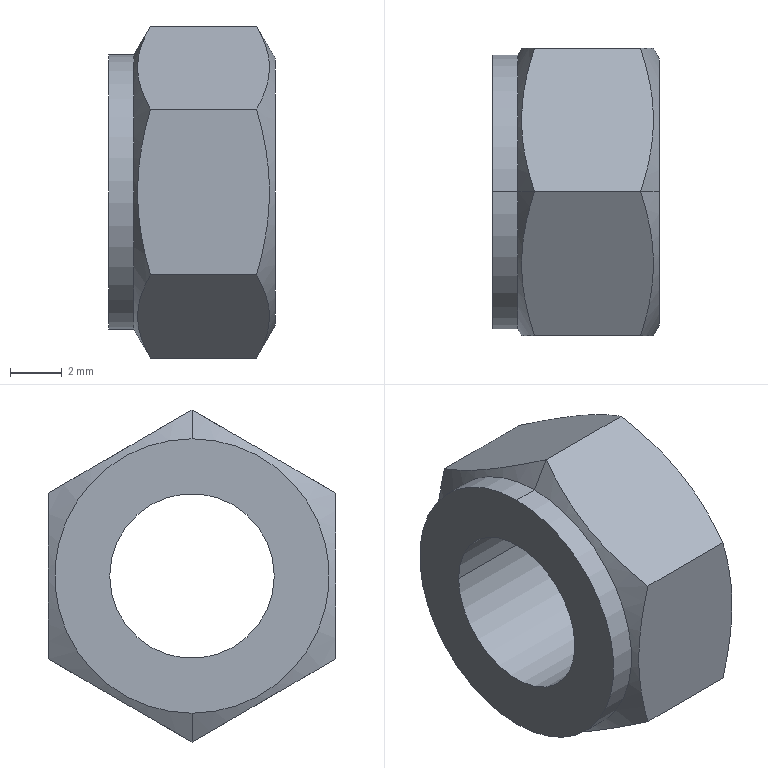Part | NX | features BREP 1 | 1 solid | 16 faces | box 6.426 x 11.1 x 12.817 mm | volume 455.339 mm3 | plane 8 | cylinder 4 | cone 4 | commonest cylinder face diameters 6.35 x2 10.592 x2
STEP:
#1=CARTESIAN_POINT('',(5.537,0.,5.159));
#2=VERTEX_POINT('',#1);
#3=CARTESIAN_POINT('',(5.537,0.,-5.159));
#4=VERTEX_POINT('',#3);
#5=CARTESIAN_POINT('',(5.537,0.,0.));
#6=DIRECTION('',(-1.,0.,0.));
#7=DIRECTION('',(0.,0.,1.));
#8=AXIS2_PLACEMENT_3D('',#5,#6,#7);
#9=CIRCLE('',#8,5.159);
#10=EDGE_CURVE('',#2,#4,#9,.T.);
#11=ORIENTED_EDGE('',*,*,#10,.F.);
#12=CARTESIAN_POINT('',(5.537,0.,0.));
#13=DIRECTION('',(-1.,0.,0.));
#14=DIRECTION('',(0.,0.,-1.));
#15=AXIS2_PLACEMENT_3D('',#12,#13,#14);
#16=CIRCLE('',#15,5.159);
#17=EDGE_CURVE('',#4,#2,#16,.T.);
#18=ORIENTED_EDGE('',*,*,#17,.F.);
#19=EDGE_LOOP('',(#11,#18));
#20=FACE_BOUND('',#19,.T.);
#21=CARTESIAN_POINT('',(5.537,-3.175,0.));
#22=VERTEX_POINT('',#21);
#23=CARTESIAN_POINT('',(5.537,3.175,0.));
#24=VERTEX_POINT('',#23);
#25=CARTESIAN_POINT('',(5.537,0.,0.));
#26=DIRECTION('',(1.,0.,0.));
#27=DIRECTION('',(0.,-1.,0.));
#28=AXIS2_PLACEMENT_3D('',#25,#26,#27);
#29=CIRCLE('',#28,3.175);
#30=EDGE_CURVE('',#22,#24,#29,.T.);
#31=ORIENTED_EDGE('',*,*,#30,.F.);
#32=CARTESIAN_POINT('',(5.537,0.,0.));
#33=DIRECTION('',(1.,0.,0.));
#34=DIRECTION('',(0.,1.,0.));
#35=AXIS2_PLACEMENT_3D('',#32,#33,#34);
#36=CIRCLE('',#35,3.175);
#37=EDGE_CURVE('',#24,#22,#36,.T.);
#38=ORIENTED_EDGE('',*,*,#37,.F.);
#39=EDGE_LOOP('',(#31,#38));
#40=FACE_BOUND('',#39,.T.);
#41=CARTESIAN_POINT('',(5.537,0.,0.));
#42=DIRECTION('',(1.,0.,0.));
#43=DIRECTION('',(0.,1.,0.));
#44=AXIS2_PLACEMENT_3D('',#41,#42,#43);
#45=PLANE('',#44);
#46=ADVANCED_FACE('',(#20,#40),#45,.T.);
#47=ORIENTED_EDGE('',*,*,#37,.T.);
#48=CARTESIAN_POINT('',(-0.889,-3.175,0.));
#49=VERTEX_POINT('',#48);
#50=CARTESIAN_POINT('',(-0.889,-3.175,0.));
#51=DIRECTION('',(1.,0.,0.));
#52=VECTOR('',#51,1000.);
#53=LINE('',#50,#52);
#54=EDGE_CURVE('',#22,#49,#53,.F.);
#55=ORIENTED_EDGE('',*,*,#54,.T.);
#56=CARTESIAN_POINT('',(-0.889,3.175,0.));
#57=VERTEX_POINT('',#56);
#58=CARTESIAN_POINT('',(-0.889,0.,0.));
#59=DIRECTION('',(1.,0.,0.));
#60=DIRECTION('',(0.,1.,0.));
#61=AXIS2_PLACEMENT_3D('',#58,#59,#60);
#62=CIRCLE('',#61,3.175);
#63=EDGE_CURVE('',#57,#49,#62,.T.);
#64=ORIENTED_EDGE('',*,*,#63,.F.);
#65=CARTESIAN_POINT('',(-0.889,3.175,0.));
#66=DIRECTION('',(1.,0.,0.));
#67=VECTOR('',#66,1000.);
#68=LINE('',#65,#67);
#69=EDGE_CURVE('',#24,#57,#68,.F.);
#70=ORIENTED_EDGE('',*,*,#69,.F.);
#71=EDGE_LOOP('',(#47,#55,#64,#70));
#72=FACE_BOUND('',#71,.T.);
#73=CARTESIAN_POINT('',(-1.532,0.,0.));
#74=DIRECTION('',(1.,0.,0.));
#75=DIRECTION('',(0.,1.,0.));
#76=AXIS2_PLACEMENT_3D('',#73,#74,#75);
#77=CYLINDRICAL_SURFACE('',#76,3.175);
#78=ADVANCED_FACE('',(#72),#77,.F.);
#79=CARTESIAN_POINT('',(-0.889,0.,0.));
#80=DIRECTION('',(1.,0.,0.));
#81=DIRECTION('',(0.,-1.,0.));
#82=AXIS2_PLACEMENT_3D('',#79,#80,#81);
#83=CIRCLE('',#82,3.175);
#84=EDGE_CURVE('',#49,#57,#83,.T.);
#85=ORIENTED_EDGE('',*,*,#84,.F.);
#86=ORIENTED_EDGE('',*,*,#54,.F.);
#87=ORIENTED_EDGE('',*,*,#30,.T.);
#88=ORIENTED_EDGE('',*,*,#69,.T.);
#89=EDGE_LOOP('',(#85,#86,#87,#88));
#90=FACE_BOUND('',#89,.T.);
#91=CARTESIAN_POINT('',(-1.532,0.,0.));
#92=DIRECTION('',(1.,0.,0.));
#93=DIRECTION('',(0.,1.,0.));
#94=AXIS2_PLACEMENT_3D('',#91,#92,#93);
#95=CYLINDRICAL_SURFACE('',#94,3.175);
#96=ADVANCED_FACE('',(#90),#95,.F.);
#97=CARTESIAN_POINT('',(-0.889,0.,5.296));
#98=VERTEX_POINT('',#97);
#99=CARTESIAN_POINT('',(-0.889,0.,-5.296));
#100=VERTEX_POINT('',#99);
#101=CARTESIAN_POINT('',(-0.889,0.,0.));
#102=DIRECTION('',(-1.,0.,0.));
#103=DIRECTION('',(0.,0.,1.));
#104=AXIS2_PLACEMENT_3D('',#101,#102,#103);
#105=CIRCLE('',#104,5.296);
#106=EDGE_CURVE('',#98,#100,#105,.T.);
#107=ORIENTED_EDGE('',*,*,#106,.T.);
#108=CARTESIAN_POINT('',(-0.889,0.,0.));
#109=DIRECTION('',(-1.,0.,0.));
#110=DIRECTION('',(0.,0.,-1.));
#111=AXIS2_PLACEMENT_3D('',#108,#109,#110);
#112=CIRCLE('',#111,5.296);
#113=EDGE_CURVE('',#100,#98,#112,.T.);
#114=ORIENTED_EDGE('',*,*,#113,.T.);
#115=EDGE_LOOP('',(#107,#114));
#116=FACE_BOUND('',#115,.T.);
#117=ORIENTED_EDGE('',*,*,#84,.T.);
#118=ORIENTED_EDGE('',*,*,#63,.T.);
#119=EDGE_LOOP('',(#117,#118));
#120=FACE_BOUND('',#119,.T.);
#121=CARTESIAN_POINT('',(-0.889,0.,0.));
#122=DIRECTION('',(-1.,0.,0.));
#123=DIRECTION('',(0.,0.,1.));
#124=AXIS2_PLACEMENT_3D('',#121,#122,#123);
#125=PLANE('',#124);
#126=ADVANCED_FACE('',(#116,#120),#125,.T.);
#127=CARTESIAN_POINT('',(0.07914,0.,5.296));
#128=VERTEX_POINT('',#127);
#129=CARTESIAN_POINT('',(0.07914,0.,5.296));
#130=DIRECTION('',(-1.,0.,0.));
#131=VECTOR('',#130,1000.);
#132=LINE('',#129,#131);
#133=EDGE_CURVE('',#98,#128,#132,.F.);
#134=ORIENTED_EDGE('',*,*,#133,.F.);
#135=ORIENTED_EDGE('',*,*,#113,.F.);
#136=CARTESIAN_POINT('',(0.07914,0.,-5.296));
#137=VERTEX_POINT('',#136);
#138=CARTESIAN_POINT('',(0.07914,0.,-5.296));
#139=DIRECTION('',(-1.,0.,0.));
#140=VECTOR('',#139,1000.);
#141=LINE('',#138,#140);
#142=EDGE_CURVE('',#100,#137,#141,.F.);
#143=ORIENTED_EDGE('',*,*,#142,.T.);
#144=CARTESIAN_POINT('',(0.07914,0.,0.));
#145=DIRECTION('',(-1.,0.,0.));
#146=DIRECTION('',(0.,0.,-1.));
#147=AXIS2_PLACEMENT_3D('',#144,#145,#146);
#148=CIRCLE('',#147,5.296);
#149=EDGE_CURVE('',#137,#128,#148,.T.);
#150=ORIENTED_EDGE('',*,*,#149,.T.);
#151=EDGE_LOOP('',(#134,#135,#143,#150));
#152=FACE_BOUND('',#151,.T.);
#153=CARTESIAN_POINT('',(0.508,0.,0.));
#154=DIRECTION('',(-1.,0.,0.));
#155=DIRECTION('',(0.,0.,-1.));
#156=AXIS2_PLACEMENT_3D('',#153,#154,#155);
#157=CYLINDRICAL_SURFACE('',#156,5.296);
#158=ADVANCED_FACE('',(#152),#157,.T.);
#159=CARTESIAN_POINT('',(0.7215,0.,-6.408));
#160=VERTEX_POINT('',#159);
#161=CARTESIAN_POINT('',(0.07914,0.,-5.296));
#162=DIRECTION('',(0.5,0.,-0.866));
#163=VECTOR('',#162,1000.);
#164=LINE('',#161,#163);
#165=EDGE_CURVE('',#137,#160,#164,.T.);
#166=ORIENTED_EDGE('',*,*,#165,.T.);
#167=CARTESIAN_POINT('',(0.7215,-5.55,-3.204));
#168=VERTEX_POINT('',#167);
#169=CARTESIAN_POINT('',(0.7215,-5.55,-3.204));
#170=CARTESIAN_POINT('',(0.06136,-3.57,-4.348));
#171=CARTESIAN_POINT('',(0.06077,-1.982,-5.264));
#172=CARTESIAN_POINT('',(0.7215,0.,-6.408));
#173=B_SPLINE_CURVE_WITH_KNOTS('',3,(#169,#170,#171,#172),.UNSPECIFIED.,.F.,.F.,(4,4),(0.,1.),.UNSPECIFIED.);
#174=EDGE_CURVE('',#160,#168,#173,.F.);
#175=ORIENTED_EDGE('',*,*,#174,.T.);
#176=CARTESIAN_POINT('',(0.7215,-5.55,3.204));
#177=VERTEX_POINT('',#176);
#178=CARTESIAN_POINT('',(0.7215,-5.55,3.204));
#179=CARTESIAN_POINT('',(0.06136,-5.55,0.9175));
#180=CARTESIAN_POINT('',(0.06077,-5.55,-0.9155));
#181=CARTESIAN_POINT('',(0.7215,-5.55,-3.204));
#182=B_SPLINE_CURVE_WITH_KNOTS('',3,(#178,#179,#180,#181),.UNSPECIFIED.,.F.,.F.,(4,4),(0.,1.),.UNSPECIFIED.);
#183=EDGE_CURVE('',#168,#177,#182,.F.);
#184=ORIENTED_EDGE('',*,*,#183,.T.);
#185=CARTESIAN_POINT('',(0.7215,0.,6.408));
#186=VERTEX_POINT('',#185);
#187=CARTESIAN_POINT('',(0.7215,0.,6.408));
#188=CARTESIAN_POINT('',(0.06136,-1.98,5.265));
#189=CARTESIAN_POINT('',(0.06077,-3.568,4.349));
#190=CARTESIAN_POINT('',(0.7215,-5.55,3.204));
#191=B_SPLINE_CURVE_WITH_KNOTS('',3,(#187,#188,#189,#190),.UNSPECIFIED.,.F.,.F.,(4,4),(0.,1.),.UNSPECIFIED.);
#192=EDGE_CURVE('',#177,#186,#191,.F.);
#193=ORIENTED_EDGE('',*,*,#192,.T.);
#194=CARTESIAN_POINT('',(0.07914,0.,5.296));
#195=DIRECTION('',(0.5,0.,0.866));
#196=VECTOR('',#195,1000.);
#197=LINE('',#194,#196);
#198=EDGE_CURVE('',#128,#186,#197,.T.);
#199=ORIENTED_EDGE('',*,*,#198,.F.);
#200=ORIENTED_EDGE('',*,*,#149,.F.);
#201=EDGE_LOOP('',(#166,#175,#184,#193,#199,#200));
#202=FACE_BOUND('',#201,.T.);
#203=CARTESIAN_POINT('',(0.4003,0.,0.));
#204=DIRECTION('',(1.,0.,0.));
#205=DIRECTION('',(0.,0.,1.));
#206=AXIS2_PLACEMENT_3D('',#203,#204,#205);
#207=CONICAL_SURFACE('',#206,5.852,1.047);
#208=ADVANCED_FACE('',(#202),#207,.T.);
#209=ORIENTED_EDGE('',*,*,#198,.T.);
#210=CARTESIAN_POINT('',(0.7215,5.55,3.204));
#211=VERTEX_POINT('',#210);
#212=CARTESIAN_POINT('',(0.7215,5.55,3.204));
#213=CARTESIAN_POINT('',(0.06136,3.57,4.348));
#214=CARTESIAN_POINT('',(0.06077,1.982,5.264));
#215=CARTESIAN_POINT('',(0.7215,0.,6.408));
#216=B_SPLINE_CURVE_WITH_KNOTS('',3,(#212,#213,#214,#215),.UNSPECIFIED.,.F.,.F.,(4,4),(0.,1.),.UNSPECIFIED.);
#217=EDGE_CURVE('',#186,#211,#216,.F.);
#218=ORIENTED_EDGE('',*,*,#217,.T.);
#219=CARTESIAN_POINT('',(0.7215,5.55,-3.204));
#220=VERTEX_POINT('',#219);
#221=CARTESIAN_POINT('',(0.7215,5.55,-3.204));
#222=CARTESIAN_POINT('',(0.06136,5.55,-0.9175));
#223=CARTESIAN_POINT('',(0.06077,5.55,0.9155));
#224=CARTESIAN_POINT('',(0.7215,5.55,3.204));
#225=B_SPLINE_CURVE_WITH_KNOTS('',3,(#221,#222,#223,#224),.UNSPECIFIED.,.F.,.F.,(4,4),(0.,1.),.UNSPECIFIED.);
#226=EDGE_CURVE('',#211,#220,#225,.F.);
#227=ORIENTED_EDGE('',*,*,#226,.T.);
#228=CARTESIAN_POINT('',(0.7215,0.,-6.408));
#229=CARTESIAN_POINT('',(0.06136,1.98,-5.265));
#230=CARTESIAN_POINT('',(0.06077,3.568,-4.349));
#231=CARTESIAN_POINT('',(0.7215,5.55,-3.204));
#232=B_SPLINE_CURVE_WITH_KNOTS('',3,(#228,#229,#230,#231),.UNSPECIFIED.,.F.,.F.,(4,4),(0.,1.),.UNSPECIFIED.);
#233=EDGE_CURVE('',#220,#160,#232,.F.);
#234=ORIENTED_EDGE('',*,*,#233,.T.);
#235=ORIENTED_EDGE('',*,*,#165,.F.);
#236=CARTESIAN_POINT('',(0.07914,0.,0.));
#237=DIRECTION('',(-1.,0.,0.));
#238=DIRECTION('',(0.,0.,1.));
#239=AXIS2_PLACEMENT_3D('',#236,#237,#238);
#240=CIRCLE('',#239,5.296);
#241=EDGE_CURVE('',#128,#137,#240,.T.);
#242=ORIENTED_EDGE('',*,*,#241,.F.);
#243=EDGE_LOOP('',(#209,#218,#227,#234,#235,#242));
#244=FACE_BOUND('',#243,.T.);
#245=CARTESIAN_POINT('',(0.4003,0.,0.));
#246=DIRECTION('',(1.,0.,0.));
#247=DIRECTION('',(0.,0.,1.));
#248=AXIS2_PLACEMENT_3D('',#245,#246,#247);
#249=CONICAL_SURFACE('',#248,5.852,1.047);
#250=ADVANCED_FACE('',(#244),#249,.T.);
#251=ORIENTED_EDGE('',*,*,#142,.F.);
#252=ORIENTED_EDGE('',*,*,#106,.F.);
#253=ORIENTED_EDGE('',*,*,#133,.T.);
#254=ORIENTED_EDGE('',*,*,#241,.T.);
#255=EDGE_LOOP('',(#251,#252,#253,#254));
#256=FACE_BOUND('',#255,.T.);
#257=CARTESIAN_POINT('',(0.508,0.,0.));
#258=DIRECTION('',(-1.,0.,0.));
#259=DIRECTION('',(0.,0.,-1.));
#260=AXIS2_PLACEMENT_3D('',#257,#258,#259);
#261=CYLINDRICAL_SURFACE('',#260,5.296);
#262=ADVANCED_FACE('',(#256),#261,.T.);
#263=CARTESIAN_POINT('',(4.816,0.,-6.408));
#264=VERTEX_POINT('',#263);
#265=CARTESIAN_POINT('',(0.7215,0.,-6.408));
#266=DIRECTION('',(1.,0.,0.));
#267=VECTOR('',#266,1000.);
#268=LINE('',#265,#267);
#269=EDGE_CURVE('',#160,#264,#268,.T.);
#270=ORIENTED_EDGE('',*,*,#269,.F.);
#271=ORIENTED_EDGE('',*,*,#233,.F.);
#272=CARTESIAN_POINT('',(4.816,5.55,-3.204));
#273=VERTEX_POINT('',#272);
#274=CARTESIAN_POINT('',(0.7215,5.55,-3.204));
#275=DIRECTION('',(1.,0.,0.));
#276=VECTOR('',#275,1000.);
#277=LINE('',#274,#276);
#278=EDGE_CURVE('',#220,#273,#277,.T.);
#279=ORIENTED_EDGE('',*,*,#278,.T.);
#280=CARTESIAN_POINT('',(4.816,5.55,-3.204));
#281=CARTESIAN_POINT('',(5.476,3.57,-4.348));
#282=CARTESIAN_POINT('',(5.477,1.982,-5.264));
#283=CARTESIAN_POINT('',(4.816,0.,-6.408));
#284=B_SPLINE_CURVE_WITH_KNOTS('',3,(#280,#281,#282,#283),.UNSPECIFIED.,.F.,.F.,(4,4),(0.,1.),.UNSPECIFIED.);
#285=EDGE_CURVE('',#273,#264,#284,.T.);
#286=ORIENTED_EDGE('',*,*,#285,.T.);
#287=EDGE_LOOP('',(#270,#271,#279,#286));
#288=FACE_BOUND('',#287,.T.);
#289=CARTESIAN_POINT('',(0.,0.,-6.408));
#290=DIRECTION('',(0.,0.5,-0.866));
#291=DIRECTION('',(-1.,0.,0.));
#292=AXIS2_PLACEMENT_3D('',#289,#290,#291);
#293=PLANE('',#292);
#294=ADVANCED_FACE('',(#288),#293,.T.);
#295=CARTESIAN_POINT('',(5.537,0.,-5.159));
#296=DIRECTION('',(-0.5,0.,-0.866));
#297=VECTOR('',#296,1000.);
#298=LINE('',#295,#297);
#299=EDGE_CURVE('',#4,#264,#298,.T.);
#300=ORIENTED_EDGE('',*,*,#299,.T.);
#301=ORIENTED_EDGE('',*,*,#285,.F.);
#302=CARTESIAN_POINT('',(4.816,5.55,3.204));
#303=VERTEX_POINT('',#302);
#304=CARTESIAN_POINT('',(4.816,5.55,3.204));
#305=CARTESIAN_POINT('',(5.476,5.55,0.9175));
#306=CARTESIAN_POINT('',(5.477,5.55,-0.9151));
#307=CARTESIAN_POINT('',(4.816,5.55,-3.204));
#308=B_SPLINE_CURVE_WITH_KNOTS('',3,(#304,#305,#306,#307),.UNSPECIFIED.,.F.,.F.,(4,4),(0.,1.),.UNSPECIFIED.);
#309=EDGE_CURVE('',#303,#273,#308,.T.);
#310=ORIENTED_EDGE('',*,*,#309,.F.);
#311=CARTESIAN_POINT('',(4.816,0.,6.408));
#312=VERTEX_POINT('',#311);
#313=CARTESIAN_POINT('',(4.816,0.,6.408));
#314=CARTESIAN_POINT('',(5.476,1.98,5.265));
#315=CARTESIAN_POINT('',(5.477,3.567,4.349));
#316=CARTESIAN_POINT('',(4.816,5.55,3.204));
#317=B_SPLINE_CURVE_WITH_KNOTS('',3,(#313,#314,#315,#316),.UNSPECIFIED.,.F.,.F.,(4,4),(0.,1.),.UNSPECIFIED.);
#318=EDGE_CURVE('',#312,#303,#317,.T.);
#319=ORIENTED_EDGE('',*,*,#318,.F.);
#320=CARTESIAN_POINT('',(5.537,0.,5.159));
#321=DIRECTION('',(-0.5,0.,0.866));
#322=VECTOR('',#321,1000.);
#323=LINE('',#320,#322);
#324=EDGE_CURVE('',#2,#312,#323,.T.);
#325=ORIENTED_EDGE('',*,*,#324,.F.);
#326=ORIENTED_EDGE('',*,*,#10,.T.);
#327=EDGE_LOOP('',(#300,#301,#310,#319,#325,#326));
#328=FACE_BOUND('',#327,.T.);
#329=CARTESIAN_POINT('',(5.176,0.,0.));
#330=DIRECTION('',(-1.,0.,0.));
#331=DIRECTION('',(0.,0.,-1.));
#332=AXIS2_PLACEMENT_3D('',#329,#330,#331);
#333=CONICAL_SURFACE('',#332,5.784,1.047);
#334=ADVANCED_FACE('',(#328),#333,.T.);
#335=ORIENTED_EDGE('',*,*,#324,.T.);
#336=CARTESIAN_POINT('',(4.816,-5.55,3.204));
#337=VERTEX_POINT('',#336);
#338=CARTESIAN_POINT('',(4.816,-5.55,3.204));
#339=CARTESIAN_POINT('',(5.476,-3.57,4.348));
#340=CARTESIAN_POINT('',(5.477,-1.982,5.264));
#341=CARTESIAN_POINT('',(4.816,0.,6.408));
#342=B_SPLINE_CURVE_WITH_KNOTS('',3,(#338,#339,#340,#341),.UNSPECIFIED.,.F.,.F.,(4,4),(0.,1.),.UNSPECIFIED.);
#343=EDGE_CURVE('',#337,#312,#342,.T.);
#344=ORIENTED_EDGE('',*,*,#343,.F.);
#345=CARTESIAN_POINT('',(4.816,-5.55,-3.204));
#346=VERTEX_POINT('',#345);
#347=CARTESIAN_POINT('',(4.816,-5.55,-3.204));
#348=CARTESIAN_POINT('',(5.476,-5.55,-0.9175));
#349=CARTESIAN_POINT('',(5.477,-5.55,0.9151));
#350=CARTESIAN_POINT('',(4.816,-5.55,3.204));
#351=B_SPLINE_CURVE_WITH_KNOTS('',3,(#347,#348,#349,#350),.UNSPECIFIED.,.F.,.F.,(4,4),(0.,1.),.UNSPECIFIED.);
#352=EDGE_CURVE('',#346,#337,#351,.T.);
#353=ORIENTED_EDGE('',*,*,#352,.F.);
#354=CARTESIAN_POINT('',(4.816,0.,-6.408));
#355=CARTESIAN_POINT('',(5.476,-1.98,-5.265));
#356=CARTESIAN_POINT('',(5.477,-3.567,-4.349));
#357=CARTESIAN_POINT('',(4.816,-5.55,-3.204));
#358=B_SPLINE_CURVE_WITH_KNOTS('',3,(#354,#355,#356,#357),.UNSPECIFIED.,.F.,.F.,(4,4),(0.,1.),.UNSPECIFIED.);
#359=EDGE_CURVE('',#264,#346,#358,.T.);
#360=ORIENTED_EDGE('',*,*,#359,.F.);
#361=ORIENTED_EDGE('',*,*,#299,.F.);
#362=ORIENTED_EDGE('',*,*,#17,.T.);
#363=EDGE_LOOP('',(#335,#344,#353,#360,#361,#362));
#364=FACE_BOUND('',#363,.T.);
#365=CARTESIAN_POINT('',(5.176,0.,0.));
#366=DIRECTION('',(-1.,0.,0.));
#367=DIRECTION('',(0.,0.,-1.));
#368=AXIS2_PLACEMENT_3D('',#365,#366,#367);
#369=CONICAL_SURFACE('',#368,5.784,1.047);
#370=ADVANCED_FACE('',(#364),#369,.T.);
#371=CARTESIAN_POINT('',(0.7215,-5.55,-3.204));
#372=DIRECTION('',(1.,0.,0.));
#373=VECTOR('',#372,1000.);
#374=LINE('',#371,#373);
#375=EDGE_CURVE('',#168,#346,#374,.T.);
#376=ORIENTED_EDGE('',*,*,#375,.F.);
#377=ORIENTED_EDGE('',*,*,#174,.F.);
#378=ORIENTED_EDGE('',*,*,#269,.T.);
#379=ORIENTED_EDGE('',*,*,#359,.T.);
#380=EDGE_LOOP('',(#376,#377,#378,#379));
#381=FACE_BOUND('',#380,.T.);
#382=CARTESIAN_POINT('',(0.,-5.55,-3.204));
#383=DIRECTION('',(0.,-0.5,-0.866));
#384=DIRECTION('',(0.,-0.866,0.5));
#385=AXIS2_PLACEMENT_3D('',#382,#383,#384);
#386=PLANE('',#385);
#387=ADVANCED_FACE('',(#381),#386,.T.);
#388=CARTESIAN_POINT('',(0.7215,-5.55,3.204));
#389=DIRECTION('',(1.,0.,0.));
#390=VECTOR('',#389,1000.);
#391=LINE('',#388,#390);
#392=EDGE_CURVE('',#177,#337,#391,.T.);
#393=ORIENTED_EDGE('',*,*,#392,.F.);
#394=ORIENTED_EDGE('',*,*,#183,.F.);
#395=ORIENTED_EDGE('',*,*,#375,.T.);
#396=ORIENTED_EDGE('',*,*,#352,.T.);
#397=EDGE_LOOP('',(#393,#394,#395,#396));
#398=FACE_BOUND('',#397,.T.);
#399=CARTESIAN_POINT('',(0.,-5.55,3.204));
#400=DIRECTION('',(0.,-1.,0.));
#401=DIRECTION('',(0.,0.,-1.));
#402=AXIS2_PLACEMENT_3D('',#399,#400,#401);
#403=PLANE('',#402);
#404=ADVANCED_FACE('',(#398),#403,.T.);
#405=CARTESIAN_POINT('',(0.7215,0.,6.408));
#406=DIRECTION('',(1.,0.,0.));
#407=VECTOR('',#406,1000.);
#408=LINE('',#405,#407);
#409=EDGE_CURVE('',#186,#312,#408,.T.);
#410=ORIENTED_EDGE('',*,*,#409,.F.);
#411=ORIENTED_EDGE('',*,*,#192,.F.);
#412=ORIENTED_EDGE('',*,*,#392,.T.);
#413=ORIENTED_EDGE('',*,*,#343,.T.);
#414=EDGE_LOOP('',(#410,#411,#412,#413));
#415=FACE_BOUND('',#414,.T.);
#416=CARTESIAN_POINT('',(0.,0.,6.408));
#417=DIRECTION('',(0.,-0.5,0.866));
#418=DIRECTION('',(-1.,0.,0.));
#419=AXIS2_PLACEMENT_3D('',#416,#417,#418);
#420=PLANE('',#419);
#421=ADVANCED_FACE('',(#415),#420,.T.);
#422=CARTESIAN_POINT('',(0.7215,5.55,3.204));
#423=DIRECTION('',(1.,0.,0.));
#424=VECTOR('',#423,1000.);
#425=LINE('',#422,#424);
#426=EDGE_CURVE('',#211,#303,#425,.T.);
#427=ORIENTED_EDGE('',*,*,#426,.F.);
#428=ORIENTED_EDGE('',*,*,#217,.F.);
#429=ORIENTED_EDGE('',*,*,#409,.T.);
#430=ORIENTED_EDGE('',*,*,#318,.T.);
#431=EDGE_LOOP('',(#427,#428,#429,#430));
#432=FACE_BOUND('',#431,.T.);
#433=CARTESIAN_POINT('',(0.,5.55,3.204));
#434=DIRECTION('',(0.,0.5,0.866));
#435=DIRECTION('',(1.,0.,0.));
#436=AXIS2_PLACEMENT_3D('',#433,#434,#435);
#437=PLANE('',#436);
#438=ADVANCED_FACE('',(#432),#437,.T.);
#439=ORIENTED_EDGE('',*,*,#278,.F.);
#440=ORIENTED_EDGE('',*,*,#226,.F.);
#441=ORIENTED_EDGE('',*,*,#426,.T.);
#442=ORIENTED_EDGE('',*,*,#309,.T.);
#443=EDGE_LOOP('',(#439,#440,#441,#442));
#444=FACE_BOUND('',#443,.T.);
#445=CARTESIAN_POINT('',(0.,5.55,-3.204));
#446=DIRECTION('',(0.,1.,0.));
#447=DIRECTION('',(1.,0.,0.));
#448=AXIS2_PLACEMENT_3D('',#445,#446,#447);
#449=PLANE('',#448);
#450=ADVANCED_FACE('',(#444),#449,.T.);
#451=CLOSED_SHELL('',(#46,#78,#96,#126,#158,#208,#250,#262,#294,#334,#370,#387,#404,#421,#438,#450));
#452=MANIFOLD_SOLID_BREP('',#451);
#453=(LENGTH_UNIT()NAMED_UNIT(*)SI_UNIT(.MILLI.,.METRE.));
#454=UNCERTAINTY_MEASURE_WITH_UNIT(LENGTH_MEASURE(0.0508),#453,'','');
#455=(NAMED_UNIT(*)PLANE_ANGLE_UNIT()SI_UNIT($,.RADIAN.));
#456=(NAMED_UNIT(*)SI_UNIT($,.STERADIAN.)SOLID_ANGLE_UNIT());
#457=(GEOMETRIC_REPRESENTATION_CONTEXT(3)GLOBAL_UNCERTAINTY_ASSIGNED_CONTEXT((#454))GLOBAL_UNIT_ASSIGNED_CONTEXT((#453,#455,#456))REPRESENTATION_CONTEXT('',''));
#458=ADVANCED_BREP_SHAPE_REPRESENTATION('',(#452),#457);